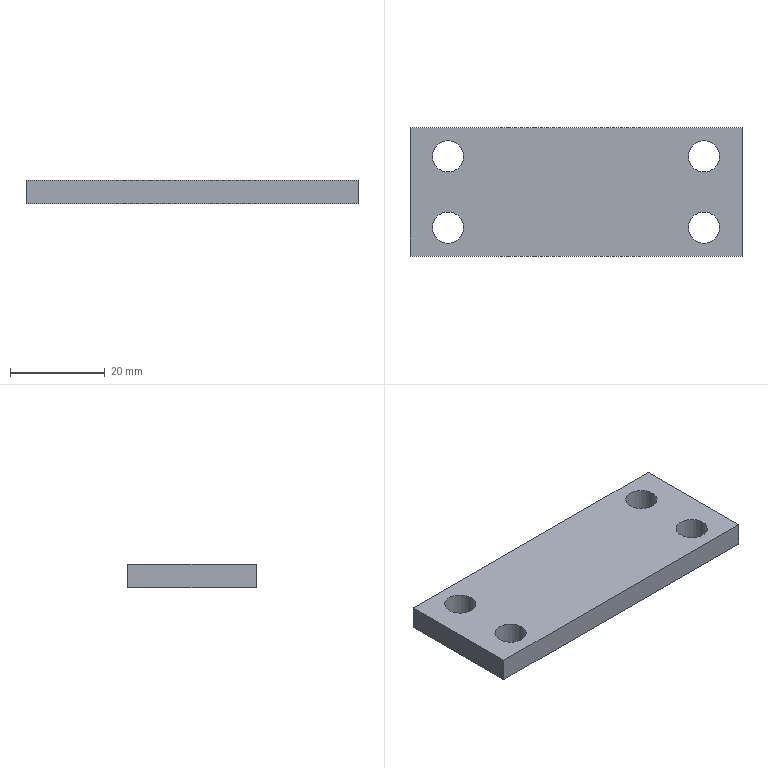Part | NX | 1 solid | 10 faces | box 70 x 27 x 5 mm | volume 8766 mm3 | plane 6 | cylinder 4 | commonest cylinder face diameters 6.6 x4
STEP:
#1=CARTESIAN_POINT('',(35.,-13.5,0.));
#2=VERTEX_POINT('',#1);
#3=CARTESIAN_POINT('',(35.,13.5,0.));
#4=VERTEX_POINT('',#3);
#5=CARTESIAN_POINT('',(35.,-13.5,0.));
#6=DIRECTION('',(0.,1.,0.));
#7=VECTOR('',#6,1000.);
#8=LINE('',#5,#7);
#9=EDGE_CURVE('',#2,#4,#8,.T.);
#10=ORIENTED_EDGE('',*,*,#9,.T.);
#11=CARTESIAN_POINT('',(35.,13.5,5.));
#12=VERTEX_POINT('',#11);
#13=CARTESIAN_POINT('',(35.,13.5,5.));
#14=DIRECTION('',(0.,0.,-1.));
#15=VECTOR('',#14,1000.);
#16=LINE('',#13,#15);
#17=EDGE_CURVE('',#12,#4,#16,.T.);
#18=ORIENTED_EDGE('',*,*,#17,.F.);
#19=CARTESIAN_POINT('',(35.,-13.5,5.));
#20=VERTEX_POINT('',#19);
#21=CARTESIAN_POINT('',(35.,-13.5,5.));
#22=DIRECTION('',(0.,1.,0.));
#23=VECTOR('',#22,1000.);
#24=LINE('',#21,#23);
#25=EDGE_CURVE('',#20,#12,#24,.T.);
#26=ORIENTED_EDGE('',*,*,#25,.F.);
#27=CARTESIAN_POINT('',(35.,-13.5,5.));
#28=DIRECTION('',(0.,0.,-1.));
#29=VECTOR('',#28,1000.);
#30=LINE('',#27,#29);
#31=EDGE_CURVE('',#20,#2,#30,.T.);
#32=ORIENTED_EDGE('',*,*,#31,.T.);
#33=EDGE_LOOP('',(#10,#18,#26,#32));
#34=FACE_BOUND('',#33,.T.);
#35=CARTESIAN_POINT('',(35.,-13.5,5.));
#36=DIRECTION('',(-1.,0.,0.));
#37=DIRECTION('',(0.,0.,1.));
#38=AXIS2_PLACEMENT_3D('',#35,#36,#37);
#39=PLANE('',#38);
#40=ADVANCED_FACE('',(#34),#39,.F.);
#41=CARTESIAN_POINT('',(-35.,13.5,0.));
#42=VERTEX_POINT('',#41);
#43=CARTESIAN_POINT('',(-35.,13.5,0.));
#44=DIRECTION('',(-1.,0.,0.));
#45=VECTOR('',#44,1000.);
#46=LINE('',#43,#45);
#47=EDGE_CURVE('',#4,#42,#46,.T.);
#48=ORIENTED_EDGE('',*,*,#47,.T.);
#49=CARTESIAN_POINT('',(-35.,13.5,5.));
#50=VERTEX_POINT('',#49);
#51=CARTESIAN_POINT('',(-35.,13.5,5.));
#52=DIRECTION('',(0.,0.,-1.));
#53=VECTOR('',#52,1000.);
#54=LINE('',#51,#53);
#55=EDGE_CURVE('',#50,#42,#54,.T.);
#56=ORIENTED_EDGE('',*,*,#55,.F.);
#57=CARTESIAN_POINT('',(-35.,13.5,5.));
#58=DIRECTION('',(-1.,0.,0.));
#59=VECTOR('',#58,1000.);
#60=LINE('',#57,#59);
#61=EDGE_CURVE('',#12,#50,#60,.T.);
#62=ORIENTED_EDGE('',*,*,#61,.F.);
#63=ORIENTED_EDGE('',*,*,#17,.T.);
#64=EDGE_LOOP('',(#48,#56,#62,#63));
#65=FACE_BOUND('',#64,.T.);
#66=CARTESIAN_POINT('',(-35.,13.5,5.));
#67=DIRECTION('',(0.,-1.,0.));
#68=DIRECTION('',(0.,0.,-1.));
#69=AXIS2_PLACEMENT_3D('',#66,#67,#68);
#70=PLANE('',#69);
#71=ADVANCED_FACE('',(#65),#70,.F.);
#72=CARTESIAN_POINT('',(-35.,-13.5,0.));
#73=VERTEX_POINT('',#72);
#74=CARTESIAN_POINT('',(-35.,-13.5,0.));
#75=DIRECTION('',(0.,-1.,0.));
#76=VECTOR('',#75,1000.);
#77=LINE('',#74,#76);
#78=EDGE_CURVE('',#42,#73,#77,.T.);
#79=ORIENTED_EDGE('',*,*,#78,.T.);
#80=CARTESIAN_POINT('',(-35.,-13.5,5.));
#81=VERTEX_POINT('',#80);
#82=CARTESIAN_POINT('',(-35.,-13.5,5.));
#83=DIRECTION('',(0.,0.,-1.));
#84=VECTOR('',#83,1000.);
#85=LINE('',#82,#84);
#86=EDGE_CURVE('',#81,#73,#85,.T.);
#87=ORIENTED_EDGE('',*,*,#86,.F.);
#88=CARTESIAN_POINT('',(-35.,-13.5,5.));
#89=DIRECTION('',(0.,-1.,0.));
#90=VECTOR('',#89,1000.);
#91=LINE('',#88,#90);
#92=EDGE_CURVE('',#50,#81,#91,.T.);
#93=ORIENTED_EDGE('',*,*,#92,.F.);
#94=ORIENTED_EDGE('',*,*,#55,.T.);
#95=EDGE_LOOP('',(#79,#87,#93,#94));
#96=FACE_BOUND('',#95,.T.);
#97=CARTESIAN_POINT('',(-35.,-13.5,5.));
#98=DIRECTION('',(1.,0.,0.));
#99=DIRECTION('',(0.,0.,-1.));
#100=AXIS2_PLACEMENT_3D('',#97,#98,#99);
#101=PLANE('',#100);
#102=ADVANCED_FACE('',(#96),#101,.F.);
#103=CARTESIAN_POINT('',(-35.,-13.5,0.));
#104=DIRECTION('',(1.,0.,0.));
#105=VECTOR('',#104,1000.);
#106=LINE('',#103,#105);
#107=EDGE_CURVE('',#73,#2,#106,.T.);
#108=ORIENTED_EDGE('',*,*,#107,.T.);
#109=ORIENTED_EDGE('',*,*,#31,.F.);
#110=CARTESIAN_POINT('',(-35.,-13.5,5.));
#111=DIRECTION('',(1.,0.,0.));
#112=VECTOR('',#111,1000.);
#113=LINE('',#110,#112);
#114=EDGE_CURVE('',#81,#20,#113,.T.);
#115=ORIENTED_EDGE('',*,*,#114,.F.);
#116=ORIENTED_EDGE('',*,*,#86,.T.);
#117=EDGE_LOOP('',(#108,#109,#115,#116));
#118=FACE_BOUND('',#117,.T.);
#119=CARTESIAN_POINT('',(-35.,-13.5,5.));
#120=DIRECTION('',(0.,1.,0.));
#121=DIRECTION('',(0.,0.,1.));
#122=AXIS2_PLACEMENT_3D('',#119,#120,#121);
#123=PLANE('',#122);
#124=ADVANCED_FACE('',(#118),#123,.F.);
#125=CARTESIAN_POINT('',(-23.7,7.5,5.));
#126=VERTEX_POINT('',#125);
#127=CARTESIAN_POINT('',(-27.,7.5,5.));
#128=DIRECTION('',(0.,0.,1.));
#129=DIRECTION('',(1.,0.,0.));
#130=AXIS2_PLACEMENT_3D('',#127,#128,#129);
#131=CIRCLE('',#130,3.3);
#132=EDGE_CURVE('',#126,#126,#131,.T.);
#133=ORIENTED_EDGE('',*,*,#132,.F.);
#134=EDGE_LOOP('',(#133));
#135=FACE_BOUND('',#134,.T.);
#136=CARTESIAN_POINT('',(30.3,7.5,5.));
#137=VERTEX_POINT('',#136);
#138=CARTESIAN_POINT('',(27.,7.5,5.));
#139=DIRECTION('',(0.,0.,1.));
#140=DIRECTION('',(1.,0.,0.));
#141=AXIS2_PLACEMENT_3D('',#138,#139,#140);
#142=CIRCLE('',#141,3.3);
#143=EDGE_CURVE('',#137,#137,#142,.T.);
#144=ORIENTED_EDGE('',*,*,#143,.F.);
#145=EDGE_LOOP('',(#144));
#146=FACE_BOUND('',#145,.T.);
#147=CARTESIAN_POINT('',(-23.7,-7.5,5.));
#148=VERTEX_POINT('',#147);
#149=CARTESIAN_POINT('',(-27.,-7.5,5.));
#150=DIRECTION('',(0.,0.,1.));
#151=DIRECTION('',(1.,0.,0.));
#152=AXIS2_PLACEMENT_3D('',#149,#150,#151);
#153=CIRCLE('',#152,3.3);
#154=EDGE_CURVE('',#148,#148,#153,.T.);
#155=ORIENTED_EDGE('',*,*,#154,.F.);
#156=EDGE_LOOP('',(#155));
#157=FACE_BOUND('',#156,.T.);
#158=CARTESIAN_POINT('',(30.3,-7.5,5.));
#159=VERTEX_POINT('',#158);
#160=CARTESIAN_POINT('',(27.,-7.5,5.));
#161=DIRECTION('',(0.,0.,1.));
#162=DIRECTION('',(1.,0.,0.));
#163=AXIS2_PLACEMENT_3D('',#160,#161,#162);
#164=CIRCLE('',#163,3.3);
#165=EDGE_CURVE('',#159,#159,#164,.T.);
#166=ORIENTED_EDGE('',*,*,#165,.F.);
#167=EDGE_LOOP('',(#166));
#168=FACE_BOUND('',#167,.T.);
#169=ORIENTED_EDGE('',*,*,#25,.T.);
#170=ORIENTED_EDGE('',*,*,#61,.T.);
#171=ORIENTED_EDGE('',*,*,#92,.T.);
#172=ORIENTED_EDGE('',*,*,#114,.T.);
#173=EDGE_LOOP('',(#169,#170,#171,#172));
#174=FACE_BOUND('',#173,.T.);
#175=CARTESIAN_POINT('',(0.,0.,5.));
#176=DIRECTION('',(0.,0.,-1.));
#177=DIRECTION('',(-1.,0.,0.));
#178=AXIS2_PLACEMENT_3D('',#175,#176,#177);
#179=PLANE('',#178);
#180=ADVANCED_FACE('',(#135,#146,#157,#168,#174),#179,.F.);
#181=CARTESIAN_POINT('',(-23.7,7.5,0.));
#182=VERTEX_POINT('',#181);
#183=CARTESIAN_POINT('',(-27.,7.5,0.));
#184=DIRECTION('',(0.,0.,1.));
#185=DIRECTION('',(1.,0.,0.));
#186=AXIS2_PLACEMENT_3D('',#183,#184,#185);
#187=CIRCLE('',#186,3.3);
#188=EDGE_CURVE('',#182,#182,#187,.T.);
#189=ORIENTED_EDGE('',*,*,#188,.T.);
#190=EDGE_LOOP('',(#189));
#191=FACE_BOUND('',#190,.T.);
#192=CARTESIAN_POINT('',(30.3,7.5,0.));
#193=VERTEX_POINT('',#192);
#194=CARTESIAN_POINT('',(27.,7.5,0.));
#195=DIRECTION('',(0.,0.,1.));
#196=DIRECTION('',(1.,0.,0.));
#197=AXIS2_PLACEMENT_3D('',#194,#195,#196);
#198=CIRCLE('',#197,3.3);
#199=EDGE_CURVE('',#193,#193,#198,.T.);
#200=ORIENTED_EDGE('',*,*,#199,.T.);
#201=EDGE_LOOP('',(#200));
#202=FACE_BOUND('',#201,.T.);
#203=CARTESIAN_POINT('',(-23.7,-7.5,0.));
#204=VERTEX_POINT('',#203);
#205=CARTESIAN_POINT('',(-27.,-7.5,0.));
#206=DIRECTION('',(0.,0.,1.));
#207=DIRECTION('',(1.,0.,0.));
#208=AXIS2_PLACEMENT_3D('',#205,#206,#207);
#209=CIRCLE('',#208,3.3);
#210=EDGE_CURVE('',#204,#204,#209,.T.);
#211=ORIENTED_EDGE('',*,*,#210,.T.);
#212=EDGE_LOOP('',(#211));
#213=FACE_BOUND('',#212,.T.);
#214=CARTESIAN_POINT('',(30.3,-7.5,0.));
#215=VERTEX_POINT('',#214);
#216=CARTESIAN_POINT('',(27.,-7.5,0.));
#217=DIRECTION('',(0.,0.,1.));
#218=DIRECTION('',(1.,0.,0.));
#219=AXIS2_PLACEMENT_3D('',#216,#217,#218);
#220=CIRCLE('',#219,3.3);
#221=EDGE_CURVE('',#215,#215,#220,.T.);
#222=ORIENTED_EDGE('',*,*,#221,.T.);
#223=EDGE_LOOP('',(#222));
#224=FACE_BOUND('',#223,.T.);
#225=ORIENTED_EDGE('',*,*,#9,.F.);
#226=ORIENTED_EDGE('',*,*,#107,.F.);
#227=ORIENTED_EDGE('',*,*,#78,.F.);
#228=ORIENTED_EDGE('',*,*,#47,.F.);
#229=EDGE_LOOP('',(#225,#226,#227,#228));
#230=FACE_BOUND('',#229,.T.);
#231=CARTESIAN_POINT('',(0.,0.,0.));
#232=DIRECTION('',(0.,0.,-1.));
#233=DIRECTION('',(-1.,0.,0.));
#234=AXIS2_PLACEMENT_3D('',#231,#232,#233);
#235=PLANE('',#234);
#236=ADVANCED_FACE('',(#191,#202,#213,#224,#230),#235,.T.);
#237=ORIENTED_EDGE('',*,*,#221,.F.);
#238=EDGE_LOOP('',(#237));
#239=FACE_BOUND('',#238,.T.);
#240=ORIENTED_EDGE('',*,*,#165,.T.);
#241=EDGE_LOOP('',(#240));
#242=FACE_BOUND('',#241,.T.);
#243=CARTESIAN_POINT('',(27.,-7.5,5.));
#244=DIRECTION('',(0.,0.,1.));
#245=DIRECTION('',(1.,0.,0.));
#246=AXIS2_PLACEMENT_3D('',#243,#244,#245);
#247=CYLINDRICAL_SURFACE('',#246,3.3);
#248=ADVANCED_FACE('',(#239,#242),#247,.F.);
#249=ORIENTED_EDGE('',*,*,#210,.F.);
#250=EDGE_LOOP('',(#249));
#251=FACE_BOUND('',#250,.T.);
#252=ORIENTED_EDGE('',*,*,#154,.T.);
#253=EDGE_LOOP('',(#252));
#254=FACE_BOUND('',#253,.T.);
#255=CARTESIAN_POINT('',(-27.,-7.5,5.));
#256=DIRECTION('',(0.,0.,1.));
#257=DIRECTION('',(1.,0.,0.));
#258=AXIS2_PLACEMENT_3D('',#255,#256,#257);
#259=CYLINDRICAL_SURFACE('',#258,3.3);
#260=ADVANCED_FACE('',(#251,#254),#259,.F.);
#261=ORIENTED_EDGE('',*,*,#199,.F.);
#262=EDGE_LOOP('',(#261));
#263=FACE_BOUND('',#262,.T.);
#264=ORIENTED_EDGE('',*,*,#143,.T.);
#265=EDGE_LOOP('',(#264));
#266=FACE_BOUND('',#265,.T.);
#267=CARTESIAN_POINT('',(27.,7.5,5.));
#268=DIRECTION('',(0.,0.,1.));
#269=DIRECTION('',(1.,0.,0.));
#270=AXIS2_PLACEMENT_3D('',#267,#268,#269);
#271=CYLINDRICAL_SURFACE('',#270,3.3);
#272=ADVANCED_FACE('',(#263,#266),#271,.F.);
#273=ORIENTED_EDGE('',*,*,#188,.F.);
#274=EDGE_LOOP('',(#273));
#275=FACE_BOUND('',#274,.T.);
#276=ORIENTED_EDGE('',*,*,#132,.T.);
#277=EDGE_LOOP('',(#276));
#278=FACE_BOUND('',#277,.T.);
#279=CARTESIAN_POINT('',(-27.,7.5,5.));
#280=DIRECTION('',(0.,0.,1.));
#281=DIRECTION('',(1.,0.,0.));
#282=AXIS2_PLACEMENT_3D('',#279,#280,#281);
#283=CYLINDRICAL_SURFACE('',#282,3.3);
#284=ADVANCED_FACE('',(#275,#278),#283,.F.);
#285=CLOSED_SHELL('',(#40,#71,#102,#124,#180,#236,#248,#260,#272,#284));
#286=MANIFOLD_SOLID_BREP('',#285);
#287=(LENGTH_UNIT()NAMED_UNIT(*)SI_UNIT(.MILLI.,.METRE.));
#288=UNCERTAINTY_MEASURE_WITH_UNIT(LENGTH_MEASURE(0.00001),#287,'','');
#289=(NAMED_UNIT(*)PLANE_ANGLE_UNIT()SI_UNIT($,.RADIAN.));
#290=(NAMED_UNIT(*)SI_UNIT($,.STERADIAN.)SOLID_ANGLE_UNIT());
#291=(GEOMETRIC_REPRESENTATION_CONTEXT(3)GLOBAL_UNCERTAINTY_ASSIGNED_CONTEXT((#288))GLOBAL_UNIT_ASSIGNED_CONTEXT((#287,#289,#290))REPRESENTATION_CONTEXT('',''));
#292=ADVANCED_BREP_SHAPE_REPRESENTATION('',(#286),#291);